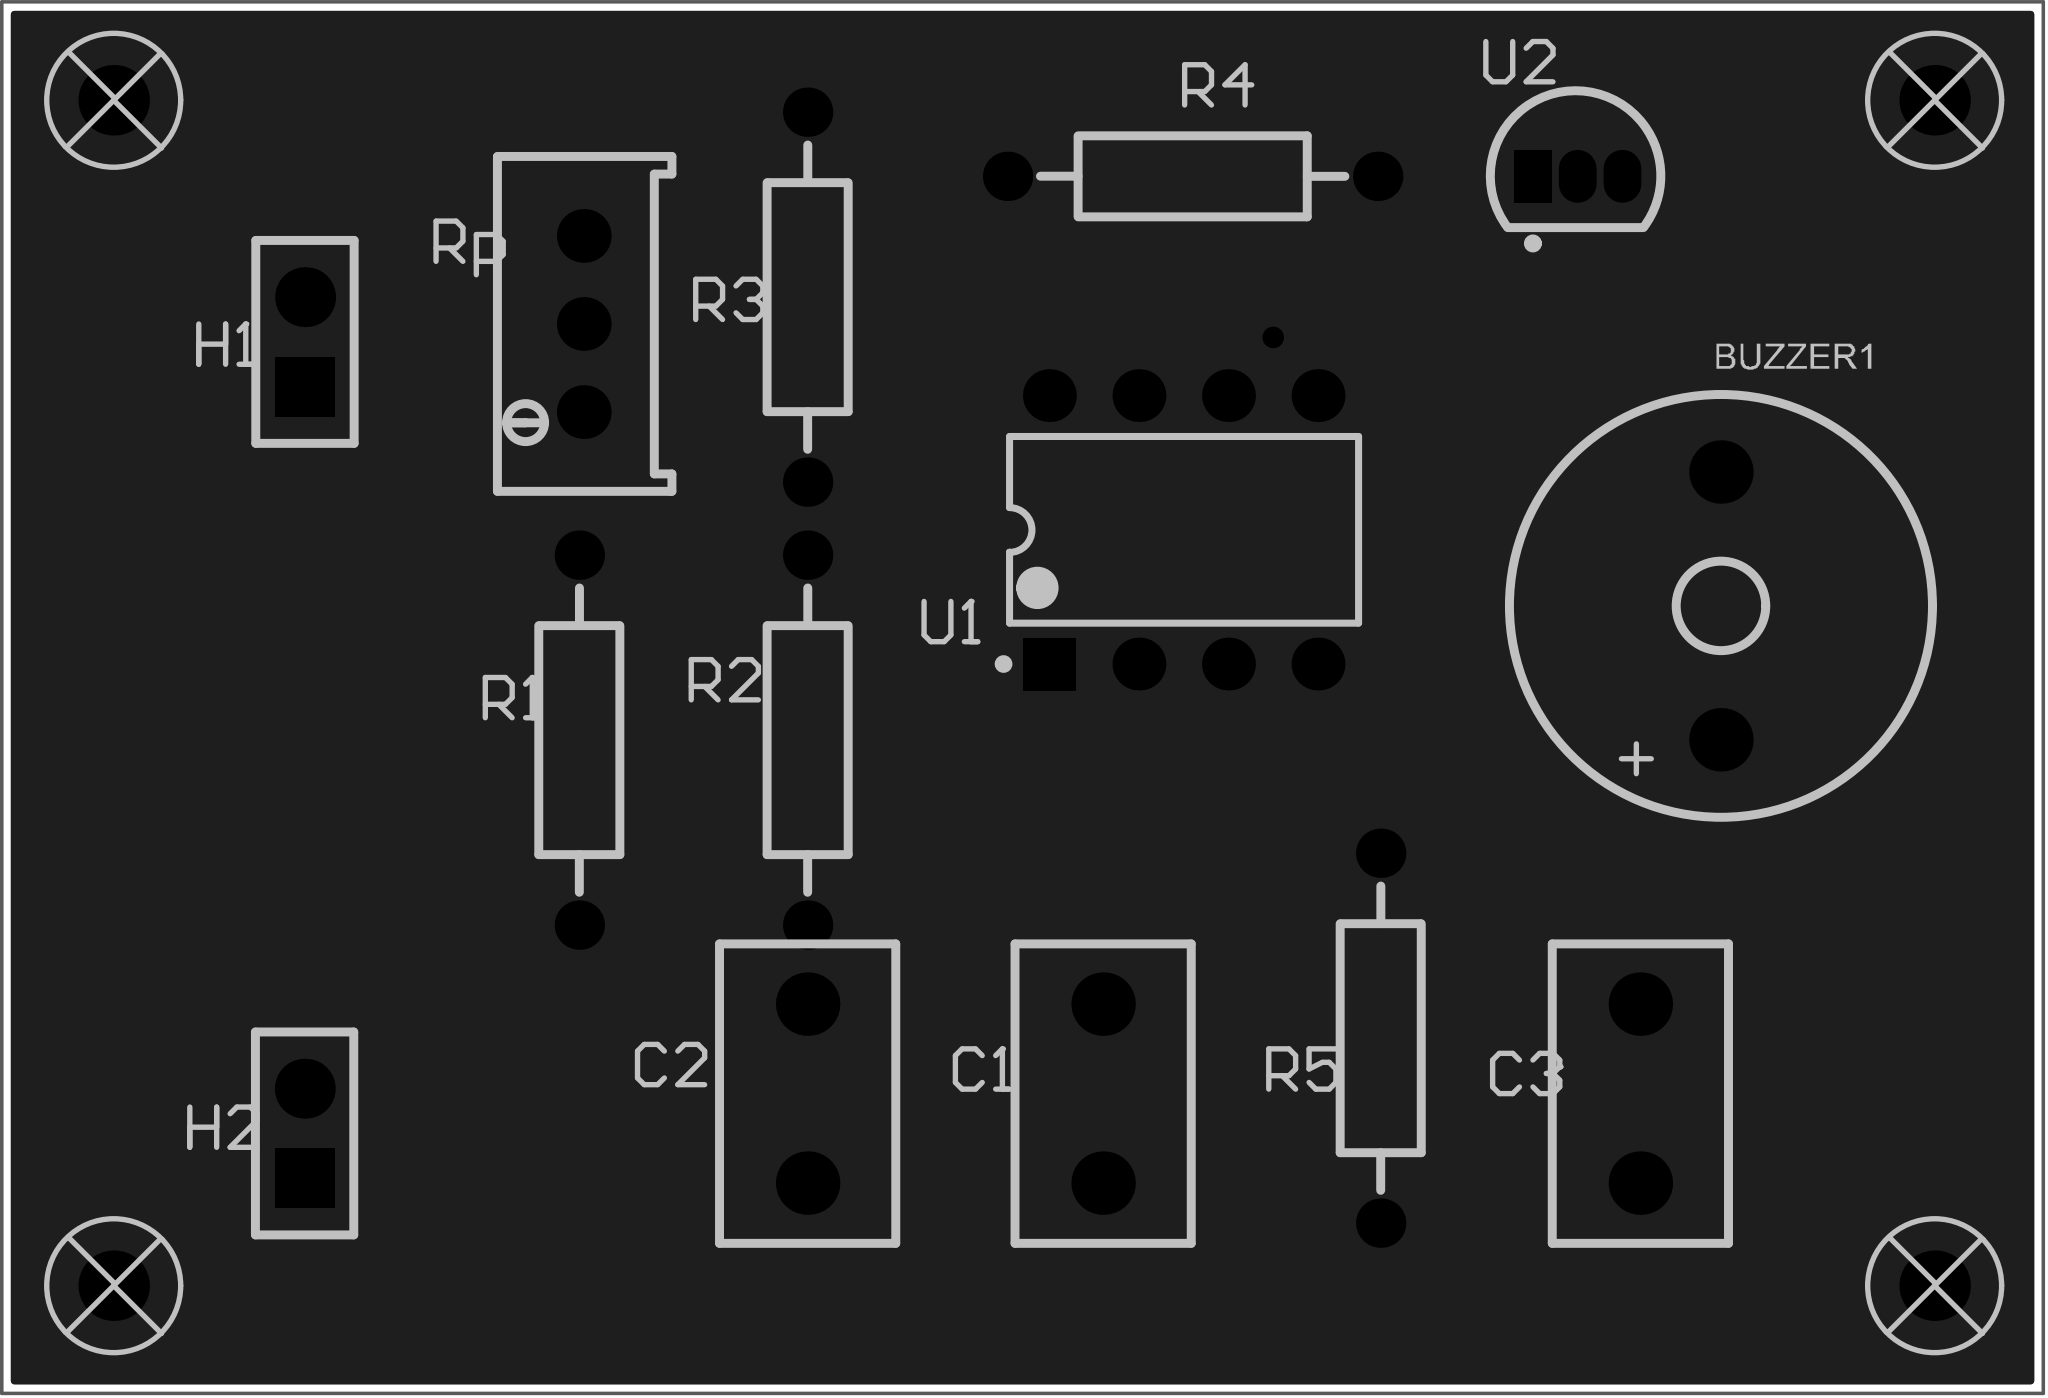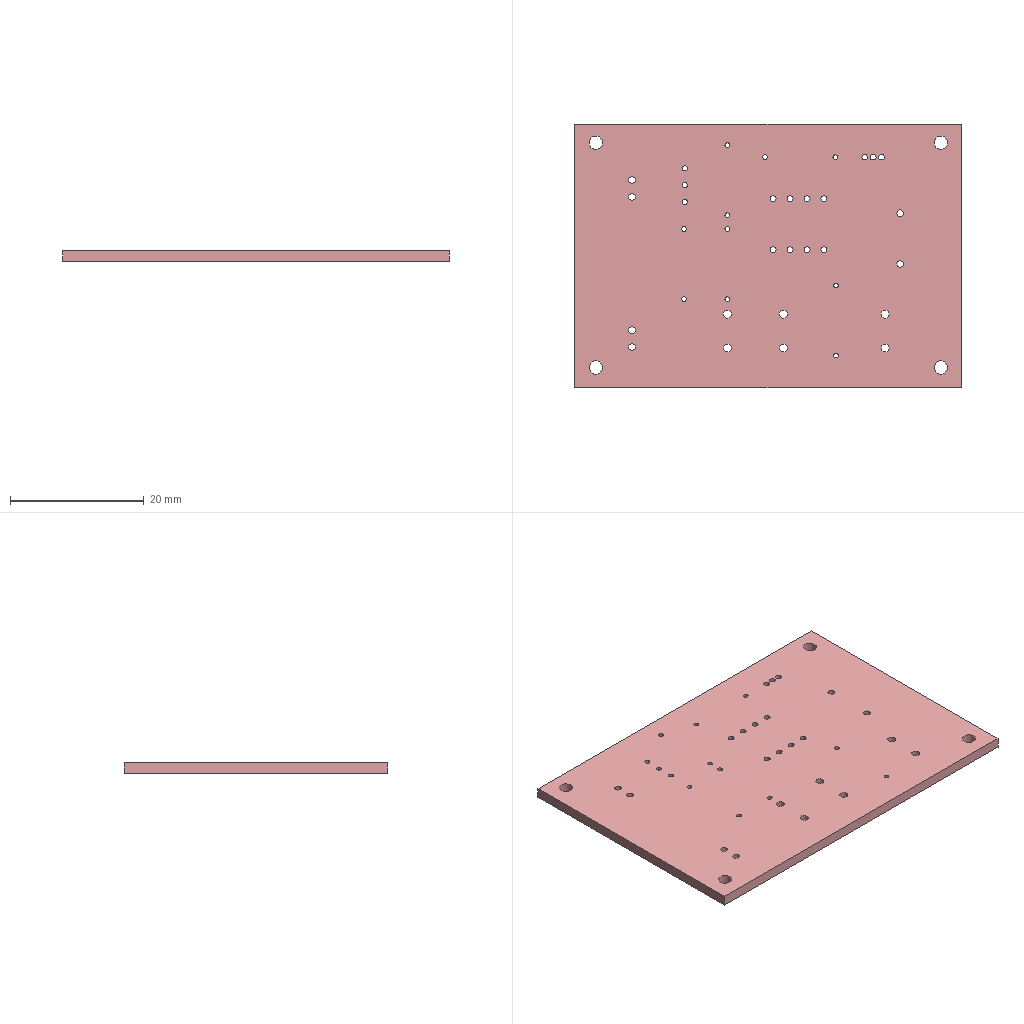Circuit board layout | Altium Designer | box 57.9 x 39.5 x 1.6 mm
Layer stack:
# Altium Designer layer stack of  (unit mm; dielectric type: 0 none, 1 core, 2 prepreg, 3 surface material)
index,name,kind,layer,copper_thickness_mm,dielectric_type,dielectric_thickness_mm,dielectric_material,dielectric_constant
0,Top Paste Mask Layer,other,,,,,,
1,Top Silkscreen Layer,other,,,,,,
2,Top Solder Mask Layer,dielectric,,,3,0.01,,3.3
3,Top Layer,copper,Top Layer,0.035,,,,
4,Dielectric1,dielectric,,,3,1.51,FR4,4.5
5,Bottom Layer,copper,Bottom Layer,0.035,,,,
6,Bottom Solder Mask Layer,dielectric,,,3,0.01,,3.3
7,Bottom Silkscreen Layer,other,,,,,,
8,Bottom Paste Mask Layer,other,,,,,,
# drill layer pairs: low layer,high layer
drill_pair,Top Layer,Bottom Layer
Part placement:
Designator,Comment,Layer,Footprint,Center-X(mm),Center-Y(mm),Rotation
U1,100kHz,TopLayer,DIP-8_L9.8-W6.6-P2.54-LS7.6-BL,110.998,101.981,0
C1,0.1uF,TopLayer,CAP-TH_L8.5-W5.0-P5.00-D1.2,108.712,85.979,270
C2,0.1uF,TopLayer,CAP-TH_L8.5-W5.0-P5.00-D1.2,100.33,85.979,90
C3,100uF,TopLayer,CAP-TH_L8.5-W5.0-P5.00-D1.2,123.952,85.979,270
H1,,TopLayer,HDR-TH_2P-P2.54-V-F,86.075,107.315,90
H2,,TopLayer,HDR-TH_2P-P2.54-V-F,86.065,84.849,90
R1,4.7kΩ,TopLayer,RES-TH_BD2.3-L6.5-P10.50-D0.5,93.853,96.012,90
R2,4.7kΩ,TopLayer,RES-TH_BD2.3-L6.5-P10.50-D0.5,100.33,96.012,90
R3,4.7kΩ,TopLayer,RES-TH_BD2.3-L6.5-P10.50-D0.5,100.33,108.585,90
R5,5.1kΩ,TopLayer,RES-TH_BD2.3-L6.5-P10.50-D0.5,116.586,87.552,90
Rp,2kΩ,TopLayer,RES-ADJ-TH_3P-L10.0-W10.0-P2.50-BL-BS,93.98,107.823,180
R4,4.7kΩ,TopLayer,RES-TH_BD2.3-L6.5-P10.50-D0.5,111.252,112.014,180
BUZZER1,,TopLayer,BUZ-TH_BD12.0-P7.60-D0.6-FD,126.238,99.822,90
SCREW1,,TopLayer,M2螺丝,80.645,114.173,0
SCREW2,,TopLayer,M2螺丝,80.645,80.527,0
SCREW3,,TopLayer,M2螺丝,132.3,80.527,0
SCREW4,,TopLayer,M2螺丝,132.3,114.173,0
U2,S9018,TopLayer,TO-92-3_L4.8-W3.7-P1.27-L,122.174,112.014,0
Pad and via stacks:
# Altium Designer via and pad stacks of  (unit mm). Each distinct definition once, with the count of objects using it.
# via: kind,start_layer,end_layer,hole_mm,diameter_mm,mode(0 simple;1 top-mid-bottom;2 full stack),diameter_per_layer,count,example_net
# pad: kind,layer,hole_mm,hole_type(0 round;1 square;2 slot),plating,top_size,top_shape(1 round;2 rect;3 octagon;9 rounded rect),mid_size,bottom_size,mode,footprint,size_per_layer,count,example
pad,Multi-Layer,0.9,0,plated,1.5x1.5,2,1.5x1.5,1.5x1.5,0,DIP-8_L9.8-W6.6-P2.54-LS7.6-BL,,1,U1.1
pad,Multi-Layer,0.9,0,plated,1.5x1.5,1,1.5x1.5,1.5x1.5,0,DIP-8_L9.8-W6.6-P2.54-LS7.6-BL,,7,U1.2
pad,Multi-Layer,1.2,0,plated,1.8x1.8,1,1.8x1.8,1.8x1.8,0,CAP-TH_L8.5-W5.0-P5.00-D1.2,,6,C1.1
pad,Multi-Layer,1,0,plated,1.7x1.7,2,1.7x1.7,1.7x1.7,0,HDR-TH_2P-P2.54-V-F,,2,H1.1
pad,Multi-Layer,1,0,plated,1.7x1.7,1,1.7x1.7,1.7x1.7,0,HDR-TH_2P-P2.54-V-F,,2,H1.2
pad,Multi-Layer,0.7,0,plated,1.4x1.4,1,1.4x1.4,1.4x1.4,0,RES-TH_BD2.3-L6.5-P10.50-D0.5,,10,R1.1
pad,Multi-Layer,0.762,0,plated,1.524x1.524,1,1.524x1.524,1.524x1.524,0,RES-ADJ-TH_3P-L10.0-W10.0-P2.50-BL-BS,,3,Rp.2
pad,Multi-Layer,1,0,plated,1.8x1.8,1,1.8x1.8,1.8x1.8,0,BUZ-TH_BD12.0-P7.60-D0.6-FD,,2,BUZZER1.2
pad,Multi-Layer,2,0,plated,2x2,1,2x2,2x2,0,M2\u00C2\u00DD\u00CB\u00BF,,4,SCREW1.1
pad,Multi-Layer,0.85,0,plated,1.07x1.5,2,1.07x1.5,1.07x1.5,0,TO-92-3_L4.8-W3.7-P1.27-L,,1,U2.1
pad,Multi-Layer,0.85,0,plated,1.07x1.5,1,1.07x1.5,1.07x1.5,0,TO-92-3_L4.8-W3.7-P1.27-L,,2,U2.2
via,Top Layer,Bottom Layer,0.3048,0.61,0,,1,$1N1510
Copper pours:
name,layer,net,type(0 solid;1 hatched;2 none)
Top Layer-GND,Top Layer,GND,0
Bottom Layer-GND,Bottom Layer,GND,0
Design rules, without the lines most boards share:
# Altium Designer design rules of  (exported by Altium Designer, unit mm)
# columns: name | kind | enabled | priority | scope1 | scope2 | descriptor | typed fields (field=value)
otherClearance | 52 | enabled | 1 | All | All | Hole To Hole Clearance (Gap=11.8mil) (All),(All) | gap=0.2997